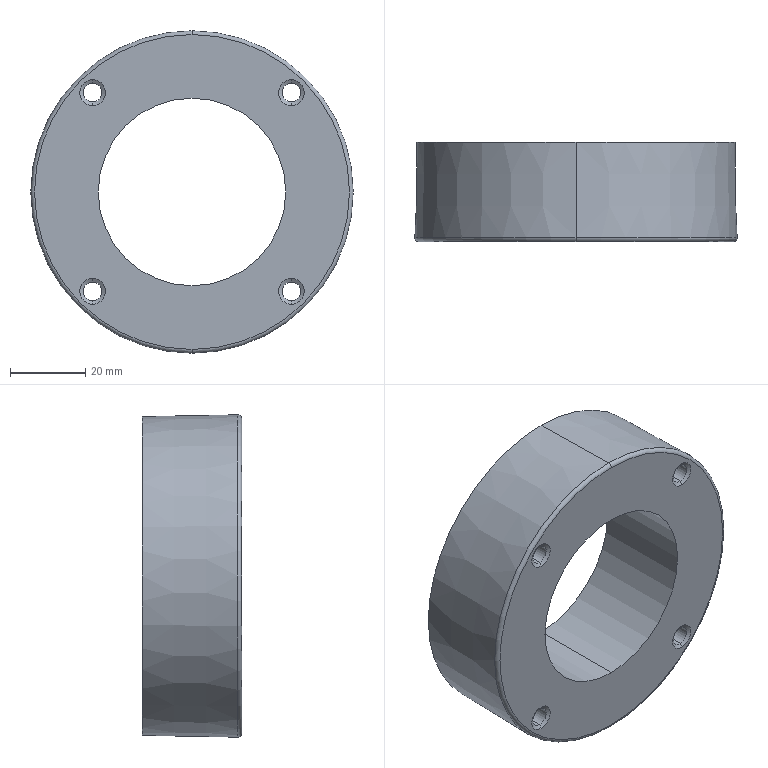Part | SolidWorks | features BaseBody 1 | 1 solid | 24 faces | box 85.962 x 26.5 x 85.962 mm | volume 97958 mm3 | cone 10 | cylinder 10 | torus 2 | plane 2 | commonest cylinder face diameters 5 x8 50 x2
STEP:
#1=CARTESIAN_POINT('',(33.,61.5,42.5));
#2=VERTEX_POINT('',#1);
#3=CARTESIAN_POINT('',(33.,61.5,-42.5));
#4=VERTEX_POINT('',#3);
#5=CARTESIAN_POINT('',(33.,61.5,0.));
#6=DIRECTION('',(0.,1.,0.));
#7=DIRECTION('',(0.,0.,-1.));
#8=AXIS2_PLACEMENT_3D('',#5,#6,#7);
#9=CIRCLE('',#8,42.5);
#10=EDGE_CURVE('',#2,#4,#9,.T.);
#11=ORIENTED_EDGE('',*,*,#10,.F.);
#12=CARTESIAN_POINT('',(33.,36.019,42.981));
#13=VERTEX_POINT('',#12);
#14=CARTESIAN_POINT('',(33.,36.019,42.981));
#15=DIRECTION('',(0.,-0.9998,0.01886));
#16=VECTOR('',#15,1000.);
#17=LINE('',#14,#16);
#18=EDGE_CURVE('',#2,#13,#17,.T.);
#19=ORIENTED_EDGE('',*,*,#18,.T.);
#20=CARTESIAN_POINT('',(33.,36.019,-42.981));
#21=VERTEX_POINT('',#20);
#22=CARTESIAN_POINT('',(33.,36.019,0.));
#23=DIRECTION('',(0.,1.,0.));
#24=DIRECTION('',(0.,0.,-1.));
#25=AXIS2_PLACEMENT_3D('',#22,#23,#24);
#26=CIRCLE('',#25,42.981);
#27=EDGE_CURVE('',#13,#21,#26,.T.);
#28=ORIENTED_EDGE('',*,*,#27,.T.);
#29=CARTESIAN_POINT('',(33.,36.019,-42.981));
#30=DIRECTION('',(0.,-0.9998,-0.01886));
#31=VECTOR('',#30,1000.);
#32=LINE('',#29,#31);
#33=EDGE_CURVE('',#4,#21,#32,.T.);
#34=ORIENTED_EDGE('',*,*,#33,.F.);
#35=EDGE_LOOP('',(#11,#19,#28,#34));
#36=FACE_OUTER_BOUND('',#35,.T.);
#37=CARTESIAN_POINT('',(33.,36.019,0.));
#38=DIRECTION('',(0.,-1.,0.));
#39=DIRECTION('',(0.,0.,-1.));
#40=AXIS2_PLACEMENT_3D('',#37,#38,#39);
#41=CONICAL_SURFACE('',#40,42.981,0.01887);
#42=ADVANCED_FACE('',(#36),#41,.T.);
#43=CARTESIAN_POINT('',(33.,61.5,25.));
#44=VERTEX_POINT('',#43);
#45=CARTESIAN_POINT('',(33.,61.5,-25.));
#46=VERTEX_POINT('',#45);
#47=CARTESIAN_POINT('',(33.,61.5,0.));
#48=DIRECTION('',(0.,-1.,0.));
#49=DIRECTION('',(0.,0.,-1.));
#50=AXIS2_PLACEMENT_3D('',#47,#48,#49);
#51=CIRCLE('',#50,25.);
#52=EDGE_CURVE('',#44,#46,#51,.T.);
#53=ORIENTED_EDGE('',*,*,#52,.F.);
#54=CARTESIAN_POINT('',(33.,35.,25.));
#55=VERTEX_POINT('',#54);
#56=CARTESIAN_POINT('',(33.,35.,25.));
#57=DIRECTION('',(0.,-1.,0.));
#58=VECTOR('',#57,1000.);
#59=LINE('',#56,#58);
#60=EDGE_CURVE('',#44,#55,#59,.T.);
#61=ORIENTED_EDGE('',*,*,#60,.T.);
#62=CARTESIAN_POINT('',(33.,35.,-25.));
#63=VERTEX_POINT('',#62);
#64=CARTESIAN_POINT('',(33.,35.,0.));
#65=DIRECTION('',(0.,1.,0.));
#66=DIRECTION('',(0.,0.,-1.));
#67=AXIS2_PLACEMENT_3D('',#64,#65,#66);
#68=CIRCLE('',#67,25.);
#69=EDGE_CURVE('',#63,#55,#68,.T.);
#70=ORIENTED_EDGE('',*,*,#69,.F.);
#71=CARTESIAN_POINT('',(33.,35.,-25.));
#72=DIRECTION('',(0.,-1.,0.));
#73=VECTOR('',#72,1000.);
#74=LINE('',#71,#73);
#75=EDGE_CURVE('',#46,#63,#74,.T.);
#76=ORIENTED_EDGE('',*,*,#75,.F.);
#77=EDGE_LOOP('',(#53,#61,#70,#76));
#78=FACE_OUTER_BOUND('',#77,.T.);
#79=CARTESIAN_POINT('',(33.,35.,0.));
#80=DIRECTION('',(0.,-1.,0.));
#81=DIRECTION('',(0.,0.,-1.));
#82=AXIS2_PLACEMENT_3D('',#79,#80,#81);
#83=CYLINDRICAL_SURFACE('',#82,25.);
#84=ADVANCED_FACE('',(#78),#83,.F.);
#85=CARTESIAN_POINT('',(59.5,61.5,29.));
#86=VERTEX_POINT('',#85);
#87=CARTESIAN_POINT('',(59.5,61.5,24.));
#88=VERTEX_POINT('',#87);
#89=CARTESIAN_POINT('',(59.5,61.5,26.5));
#90=DIRECTION('',(0.,-1.,0.));
#91=DIRECTION('',(0.,0.,-1.));
#92=AXIS2_PLACEMENT_3D('',#89,#90,#91);
#93=CIRCLE('',#92,2.5);
#94=EDGE_CURVE('',#86,#88,#93,.T.);
#95=ORIENTED_EDGE('',*,*,#94,.F.);
#96=CARTESIAN_POINT('',(59.5,35.548,29.));
#97=VERTEX_POINT('',#96);
#98=CARTESIAN_POINT('',(59.5,35.,29.));
#99=DIRECTION('',(0.,-1.,0.));
#100=VECTOR('',#99,1000.);
#101=LINE('',#98,#100);
#102=EDGE_CURVE('',#86,#97,#101,.T.);
#103=ORIENTED_EDGE('',*,*,#102,.T.);
#104=CARTESIAN_POINT('',(59.5,35.548,24.));
#105=VERTEX_POINT('',#104);
#106=CARTESIAN_POINT('',(59.5,35.548,26.5));
#107=DIRECTION('',(0.,1.,0.));
#108=DIRECTION('',(0.,0.,-1.));
#109=AXIS2_PLACEMENT_3D('',#106,#107,#108);
#110=CIRCLE('',#109,2.5);
#111=EDGE_CURVE('',#105,#97,#110,.T.);
#112=ORIENTED_EDGE('',*,*,#111,.F.);
#113=CARTESIAN_POINT('',(59.5,35.,24.));
#114=DIRECTION('',(0.,-1.,0.));
#115=VECTOR('',#114,1000.);
#116=LINE('',#113,#115);
#117=EDGE_CURVE('',#88,#105,#116,.T.);
#118=ORIENTED_EDGE('',*,*,#117,.F.);
#119=EDGE_LOOP('',(#95,#103,#112,#118));
#120=FACE_OUTER_BOUND('',#119,.T.);
#121=CARTESIAN_POINT('',(59.5,35.,26.5));
#122=DIRECTION('',(0.,-1.,0.));
#123=DIRECTION('',(0.,0.,-1.));
#124=AXIS2_PLACEMENT_3D('',#121,#122,#123);
#125=CYLINDRICAL_SURFACE('',#124,2.5);
#126=ADVANCED_FACE('',(#120),#125,.F.);
#127=CARTESIAN_POINT('',(59.5,61.5,-24.));
#128=VERTEX_POINT('',#127);
#129=CARTESIAN_POINT('',(59.5,61.5,-29.));
#130=VERTEX_POINT('',#129);
#131=CARTESIAN_POINT('',(59.5,61.5,-26.5));
#132=DIRECTION('',(0.,-1.,0.));
#133=DIRECTION('',(0.,0.,-1.));
#134=AXIS2_PLACEMENT_3D('',#131,#132,#133);
#135=CIRCLE('',#134,2.5);
#136=EDGE_CURVE('',#128,#130,#135,.T.);
#137=ORIENTED_EDGE('',*,*,#136,.F.);
#138=CARTESIAN_POINT('',(59.5,35.548,-24.));
#139=VERTEX_POINT('',#138);
#140=CARTESIAN_POINT('',(59.5,35.,-24.));
#141=DIRECTION('',(0.,-1.,0.));
#142=VECTOR('',#141,1000.);
#143=LINE('',#140,#142);
#144=EDGE_CURVE('',#128,#139,#143,.T.);
#145=ORIENTED_EDGE('',*,*,#144,.T.);
#146=CARTESIAN_POINT('',(59.5,35.548,-29.));
#147=VERTEX_POINT('',#146);
#148=CARTESIAN_POINT('',(59.5,35.548,-26.5));
#149=DIRECTION('',(0.,1.,0.));
#150=DIRECTION('',(0.,0.,-1.));
#151=AXIS2_PLACEMENT_3D('',#148,#149,#150);
#152=CIRCLE('',#151,2.5);
#153=EDGE_CURVE('',#147,#139,#152,.T.);
#154=ORIENTED_EDGE('',*,*,#153,.F.);
#155=CARTESIAN_POINT('',(59.5,35.,-29.));
#156=DIRECTION('',(0.,-1.,0.));
#157=VECTOR('',#156,1000.);
#158=LINE('',#155,#157);
#159=EDGE_CURVE('',#130,#147,#158,.T.);
#160=ORIENTED_EDGE('',*,*,#159,.F.);
#161=EDGE_LOOP('',(#137,#145,#154,#160));
#162=FACE_OUTER_BOUND('',#161,.T.);
#163=CARTESIAN_POINT('',(59.5,35.,-26.5));
#164=DIRECTION('',(0.,-1.,0.));
#165=DIRECTION('',(0.,0.,-1.));
#166=AXIS2_PLACEMENT_3D('',#163,#164,#165);
#167=CYLINDRICAL_SURFACE('',#166,2.5);
#168=ADVANCED_FACE('',(#162),#167,.F.);
#169=CARTESIAN_POINT('',(6.5,61.5,-24.));
#170=VERTEX_POINT('',#169);
#171=CARTESIAN_POINT('',(6.5,61.5,-29.));
#172=VERTEX_POINT('',#171);
#173=CARTESIAN_POINT('',(6.5,61.5,-26.5));
#174=DIRECTION('',(0.,-1.,0.));
#175=DIRECTION('',(0.,0.,-1.));
#176=AXIS2_PLACEMENT_3D('',#173,#174,#175);
#177=CIRCLE('',#176,2.5);
#178=EDGE_CURVE('',#170,#172,#177,.T.);
#179=ORIENTED_EDGE('',*,*,#178,.F.);
#180=CARTESIAN_POINT('',(6.5,35.548,-24.));
#181=VERTEX_POINT('',#180);
#182=CARTESIAN_POINT('',(6.5,35.,-24.));
#183=DIRECTION('',(0.,-1.,0.));
#184=VECTOR('',#183,1000.);
#185=LINE('',#182,#184);
#186=EDGE_CURVE('',#170,#181,#185,.T.);
#187=ORIENTED_EDGE('',*,*,#186,.T.);
#188=CARTESIAN_POINT('',(6.5,35.548,-29.));
#189=VERTEX_POINT('',#188);
#190=CARTESIAN_POINT('',(6.5,35.548,-26.5));
#191=DIRECTION('',(0.,1.,0.));
#192=DIRECTION('',(0.,0.,-1.));
#193=AXIS2_PLACEMENT_3D('',#190,#191,#192);
#194=CIRCLE('',#193,2.5);
#195=EDGE_CURVE('',#189,#181,#194,.T.);
#196=ORIENTED_EDGE('',*,*,#195,.F.);
#197=CARTESIAN_POINT('',(6.5,35.,-29.));
#198=DIRECTION('',(0.,-1.,0.));
#199=VECTOR('',#198,1000.);
#200=LINE('',#197,#199);
#201=EDGE_CURVE('',#172,#189,#200,.T.);
#202=ORIENTED_EDGE('',*,*,#201,.F.);
#203=EDGE_LOOP('',(#179,#187,#196,#202));
#204=FACE_OUTER_BOUND('',#203,.T.);
#205=CARTESIAN_POINT('',(6.5,35.,-26.5));
#206=DIRECTION('',(0.,-1.,0.));
#207=DIRECTION('',(0.,0.,-1.));
#208=AXIS2_PLACEMENT_3D('',#205,#206,#207);
#209=CYLINDRICAL_SURFACE('',#208,2.5);
#210=ADVANCED_FACE('',(#204),#209,.F.);
#211=CARTESIAN_POINT('',(6.5,61.5,29.));
#212=VERTEX_POINT('',#211);
#213=CARTESIAN_POINT('',(6.5,61.5,24.));
#214=VERTEX_POINT('',#213);
#215=CARTESIAN_POINT('',(6.5,61.5,26.5));
#216=DIRECTION('',(0.,-1.,0.));
#217=DIRECTION('',(0.,0.,-1.));
#218=AXIS2_PLACEMENT_3D('',#215,#216,#217);
#219=CIRCLE('',#218,2.5);
#220=EDGE_CURVE('',#212,#214,#219,.T.);
#221=ORIENTED_EDGE('',*,*,#220,.F.);
#222=CARTESIAN_POINT('',(6.5,35.548,29.));
#223=VERTEX_POINT('',#222);
#224=CARTESIAN_POINT('',(6.5,35.,29.));
#225=DIRECTION('',(0.,-1.,0.));
#226=VECTOR('',#225,1000.);
#227=LINE('',#224,#226);
#228=EDGE_CURVE('',#212,#223,#227,.T.);
#229=ORIENTED_EDGE('',*,*,#228,.T.);
#230=CARTESIAN_POINT('',(6.5,35.548,24.));
#231=VERTEX_POINT('',#230);
#232=CARTESIAN_POINT('',(6.5,35.548,26.5));
#233=DIRECTION('',(0.,1.,0.));
#234=DIRECTION('',(0.,0.,-1.));
#235=AXIS2_PLACEMENT_3D('',#232,#233,#234);
#236=CIRCLE('',#235,2.5);
#237=EDGE_CURVE('',#231,#223,#236,.T.);
#238=ORIENTED_EDGE('',*,*,#237,.F.);
#239=CARTESIAN_POINT('',(6.5,35.,24.));
#240=DIRECTION('',(0.,-1.,0.));
#241=VECTOR('',#240,1000.);
#242=LINE('',#239,#241);
#243=EDGE_CURVE('',#214,#231,#242,.T.);
#244=ORIENTED_EDGE('',*,*,#243,.F.);
#245=EDGE_LOOP('',(#221,#229,#238,#244));
#246=FACE_OUTER_BOUND('',#245,.T.);
#247=CARTESIAN_POINT('',(6.5,35.,26.5));
#248=DIRECTION('',(0.,-1.,0.));
#249=DIRECTION('',(0.,0.,-1.));
#250=AXIS2_PLACEMENT_3D('',#247,#248,#249);
#251=CYLINDRICAL_SURFACE('',#250,2.5);
#252=ADVANCED_FACE('',(#246),#251,.F.);
#253=ORIENTED_EDGE('',*,*,#27,.F.);
#254=CARTESIAN_POINT('',(33.,35.,41.981));
#255=VERTEX_POINT('',#254);
#256=CARTESIAN_POINT('',(33.,36.,41.981));
#257=DIRECTION('',(1.,0.,0.));
#258=DIRECTION('',(0.,0.,-1.));
#259=AXIS2_PLACEMENT_3D('',#256,#257,#258);
#260=CIRCLE('',#259,1.);
#261=EDGE_CURVE('',#13,#255,#260,.T.);
#262=ORIENTED_EDGE('',*,*,#261,.T.);
#263=CARTESIAN_POINT('',(33.,35.,-41.981));
#264=VERTEX_POINT('',#263);
#265=CARTESIAN_POINT('',(33.,35.,0.));
#266=DIRECTION('',(0.,1.,0.));
#267=DIRECTION('',(0.,0.,-1.));
#268=AXIS2_PLACEMENT_3D('',#265,#266,#267);
#269=CIRCLE('',#268,41.981);
#270=EDGE_CURVE('',#255,#264,#269,.T.);
#271=ORIENTED_EDGE('',*,*,#270,.T.);
#272=CARTESIAN_POINT('',(33.,36.,-41.981));
#273=DIRECTION('',(-1.,0.,0.));
#274=DIRECTION('',(0.,0.,1.));
#275=AXIS2_PLACEMENT_3D('',#272,#273,#274);
#276=CIRCLE('',#275,1.);
#277=EDGE_CURVE('',#21,#264,#276,.T.);
#278=ORIENTED_EDGE('',*,*,#277,.F.);
#279=EDGE_LOOP('',(#253,#262,#271,#278));
#280=FACE_OUTER_BOUND('',#279,.T.);
#281=CARTESIAN_POINT('',(33.,36.,0.));
#282=DIRECTION('',(0.,-1.,0.));
#283=DIRECTION('',(0.,0.,-1.));
#284=AXIS2_PLACEMENT_3D('',#281,#282,#283);
#285=TOROIDAL_SURFACE('',#284,41.981,1.);
#286=ADVANCED_FACE('',(#280),#285,.T.);
#287=ORIENTED_EDGE('',*,*,#111,.T.);
#288=CARTESIAN_POINT('',(59.5,35.,29.95));
#289=VERTEX_POINT('',#288);
#290=CARTESIAN_POINT('',(59.5,35.,29.95));
#291=DIRECTION('',(0.,-0.5,0.866));
#292=VECTOR('',#291,1000.);
#293=LINE('',#290,#292);
#294=EDGE_CURVE('',#97,#289,#293,.T.);
#295=ORIENTED_EDGE('',*,*,#294,.T.);
#296=CARTESIAN_POINT('',(59.5,35.,23.05));
#297=VERTEX_POINT('',#296);
#298=CARTESIAN_POINT('',(59.5,35.,26.5));
#299=DIRECTION('',(0.,-1.,0.));
#300=DIRECTION('',(0.,0.,-1.));
#301=AXIS2_PLACEMENT_3D('',#298,#299,#300);
#302=CIRCLE('',#301,3.45);
#303=EDGE_CURVE('',#289,#297,#302,.T.);
#304=ORIENTED_EDGE('',*,*,#303,.T.);
#305=CARTESIAN_POINT('',(59.5,35.,23.05));
#306=DIRECTION('',(0.,-0.5,-0.866));
#307=VECTOR('',#306,1000.);
#308=LINE('',#305,#307);
#309=EDGE_CURVE('',#105,#297,#308,.T.);
#310=ORIENTED_EDGE('',*,*,#309,.F.);
#311=EDGE_LOOP('',(#287,#295,#304,#310));
#312=FACE_OUTER_BOUND('',#311,.T.);
#313=CARTESIAN_POINT('',(59.5,35.,26.5));
#314=DIRECTION('',(0.,-1.,0.));
#315=DIRECTION('',(0.,0.,-1.));
#316=AXIS2_PLACEMENT_3D('',#313,#314,#315);
#317=CONICAL_SURFACE('',#316,3.45,1.047);
#318=ADVANCED_FACE('',(#312),#317,.F.);
#319=ORIENTED_EDGE('',*,*,#153,.T.);
#320=CARTESIAN_POINT('',(59.5,35.,-23.05));
#321=VERTEX_POINT('',#320);
#322=CARTESIAN_POINT('',(59.5,35.,-23.05));
#323=DIRECTION('',(0.,-0.5,0.866));
#324=VECTOR('',#323,1000.);
#325=LINE('',#322,#324);
#326=EDGE_CURVE('',#139,#321,#325,.T.);
#327=ORIENTED_EDGE('',*,*,#326,.T.);
#328=CARTESIAN_POINT('',(59.5,35.,-29.95));
#329=VERTEX_POINT('',#328);
#330=CARTESIAN_POINT('',(59.5,35.,-26.5));
#331=DIRECTION('',(0.,-1.,0.));
#332=DIRECTION('',(0.,0.,-1.));
#333=AXIS2_PLACEMENT_3D('',#330,#331,#332);
#334=CIRCLE('',#333,3.45);
#335=EDGE_CURVE('',#321,#329,#334,.T.);
#336=ORIENTED_EDGE('',*,*,#335,.T.);
#337=CARTESIAN_POINT('',(59.5,35.,-29.95));
#338=DIRECTION('',(0.,-0.5,-0.866));
#339=VECTOR('',#338,1000.);
#340=LINE('',#337,#339);
#341=EDGE_CURVE('',#147,#329,#340,.T.);
#342=ORIENTED_EDGE('',*,*,#341,.F.);
#343=EDGE_LOOP('',(#319,#327,#336,#342));
#344=FACE_OUTER_BOUND('',#343,.T.);
#345=CARTESIAN_POINT('',(59.5,35.,-26.5));
#346=DIRECTION('',(0.,-1.,0.));
#347=DIRECTION('',(0.,0.,-1.));
#348=AXIS2_PLACEMENT_3D('',#345,#346,#347);
#349=CONICAL_SURFACE('',#348,3.45,1.047);
#350=ADVANCED_FACE('',(#344),#349,.F.);
#351=ORIENTED_EDGE('',*,*,#195,.T.);
#352=CARTESIAN_POINT('',(6.5,35.,-23.05));
#353=VERTEX_POINT('',#352);
#354=CARTESIAN_POINT('',(6.5,35.,-23.05));
#355=DIRECTION('',(0.,-0.5,0.866));
#356=VECTOR('',#355,1000.);
#357=LINE('',#354,#356);
#358=EDGE_CURVE('',#181,#353,#357,.T.);
#359=ORIENTED_EDGE('',*,*,#358,.T.);
#360=CARTESIAN_POINT('',(6.5,35.,-29.95));
#361=VERTEX_POINT('',#360);
#362=CARTESIAN_POINT('',(6.5,35.,-26.5));
#363=DIRECTION('',(0.,-1.,0.));
#364=DIRECTION('',(0.,0.,-1.));
#365=AXIS2_PLACEMENT_3D('',#362,#363,#364);
#366=CIRCLE('',#365,3.45);
#367=EDGE_CURVE('',#353,#361,#366,.T.);
#368=ORIENTED_EDGE('',*,*,#367,.T.);
#369=CARTESIAN_POINT('',(6.5,35.,-29.95));
#370=DIRECTION('',(0.,-0.5,-0.866));
#371=VECTOR('',#370,1000.);
#372=LINE('',#369,#371);
#373=EDGE_CURVE('',#189,#361,#372,.T.);
#374=ORIENTED_EDGE('',*,*,#373,.F.);
#375=EDGE_LOOP('',(#351,#359,#368,#374));
#376=FACE_OUTER_BOUND('',#375,.T.);
#377=CARTESIAN_POINT('',(6.5,35.,-26.5));
#378=DIRECTION('',(0.,-1.,0.));
#379=DIRECTION('',(0.,0.,-1.));
#380=AXIS2_PLACEMENT_3D('',#377,#378,#379);
#381=CONICAL_SURFACE('',#380,3.45,1.047);
#382=ADVANCED_FACE('',(#376),#381,.F.);
#383=ORIENTED_EDGE('',*,*,#237,.T.);
#384=CARTESIAN_POINT('',(6.5,35.,29.95));
#385=VERTEX_POINT('',#384);
#386=CARTESIAN_POINT('',(6.5,35.,29.95));
#387=DIRECTION('',(0.,-0.5,0.866));
#388=VECTOR('',#387,1000.);
#389=LINE('',#386,#388);
#390=EDGE_CURVE('',#223,#385,#389,.T.);
#391=ORIENTED_EDGE('',*,*,#390,.T.);
#392=CARTESIAN_POINT('',(6.5,35.,23.05));
#393=VERTEX_POINT('',#392);
#394=CARTESIAN_POINT('',(6.5,35.,26.5));
#395=DIRECTION('',(0.,-1.,0.));
#396=DIRECTION('',(0.,0.,-1.));
#397=AXIS2_PLACEMENT_3D('',#394,#395,#396);
#398=CIRCLE('',#397,3.45);
#399=EDGE_CURVE('',#385,#393,#398,.T.);
#400=ORIENTED_EDGE('',*,*,#399,.T.);
#401=CARTESIAN_POINT('',(6.5,35.,23.05));
#402=DIRECTION('',(0.,-0.5,-0.866));
#403=VECTOR('',#402,1000.);
#404=LINE('',#401,#403);
#405=EDGE_CURVE('',#231,#393,#404,.T.);
#406=ORIENTED_EDGE('',*,*,#405,.F.);
#407=EDGE_LOOP('',(#383,#391,#400,#406));
#408=FACE_OUTER_BOUND('',#407,.T.);
#409=CARTESIAN_POINT('',(6.5,35.,26.5));
#410=DIRECTION('',(0.,-1.,0.));
#411=DIRECTION('',(0.,0.,-1.));
#412=AXIS2_PLACEMENT_3D('',#409,#410,#411);
#413=CONICAL_SURFACE('',#412,3.45,1.047);
#414=ADVANCED_FACE('',(#408),#413,.F.);
#415=CARTESIAN_POINT('',(33.,61.5,0.));
#416=DIRECTION('',(0.,1.,0.));
#417=DIRECTION('',(0.,0.,-1.));
#418=AXIS2_PLACEMENT_3D('',#415,#416,#417);
#419=CIRCLE('',#418,42.5);
#420=EDGE_CURVE('',#4,#2,#419,.T.);
#421=ORIENTED_EDGE('',*,*,#420,.T.);
#422=ORIENTED_EDGE('',*,*,#10,.T.);
#423=EDGE_LOOP('',(#421,#422));
#424=FACE_OUTER_BOUND('',#423,.T.);
#425=CARTESIAN_POINT('',(33.,61.5,0.));
#426=DIRECTION('',(0.,-1.,0.));
#427=DIRECTION('',(0.,0.,-1.));
#428=AXIS2_PLACEMENT_3D('',#425,#426,#427);
#429=CIRCLE('',#428,25.);
#430=EDGE_CURVE('',#46,#44,#429,.T.);
#431=ORIENTED_EDGE('',*,*,#430,.T.);
#432=ORIENTED_EDGE('',*,*,#52,.T.);
#433=EDGE_LOOP('',(#431,#432));
#434=FACE_BOUND('',#433,.T.);
#435=CARTESIAN_POINT('',(59.5,61.5,26.5));
#436=DIRECTION('',(0.,-1.,0.));
#437=DIRECTION('',(0.,0.,-1.));
#438=AXIS2_PLACEMENT_3D('',#435,#436,#437);
#439=CIRCLE('',#438,2.5);
#440=EDGE_CURVE('',#88,#86,#439,.T.);
#441=ORIENTED_EDGE('',*,*,#440,.T.);
#442=ORIENTED_EDGE('',*,*,#94,.T.);
#443=EDGE_LOOP('',(#441,#442));
#444=FACE_BOUND('',#443,.T.);
#445=CARTESIAN_POINT('',(59.5,61.5,-26.5));
#446=DIRECTION('',(0.,-1.,0.));
#447=DIRECTION('',(0.,0.,-1.));
#448=AXIS2_PLACEMENT_3D('',#445,#446,#447);
#449=CIRCLE('',#448,2.5);
#450=EDGE_CURVE('',#130,#128,#449,.T.);
#451=ORIENTED_EDGE('',*,*,#450,.T.);
#452=ORIENTED_EDGE('',*,*,#136,.T.);
#453=EDGE_LOOP('',(#451,#452));
#454=FACE_BOUND('',#453,.T.);
#455=CARTESIAN_POINT('',(6.5,61.5,-26.5));
#456=DIRECTION('',(0.,-1.,0.));
#457=DIRECTION('',(0.,0.,-1.));
#458=AXIS2_PLACEMENT_3D('',#455,#456,#457);
#459=CIRCLE('',#458,2.5);
#460=EDGE_CURVE('',#172,#170,#459,.T.);
#461=ORIENTED_EDGE('',*,*,#460,.T.);
#462=ORIENTED_EDGE('',*,*,#178,.T.);
#463=EDGE_LOOP('',(#461,#462));
#464=FACE_BOUND('',#463,.T.);
#465=CARTESIAN_POINT('',(6.5,61.5,26.5));
#466=DIRECTION('',(0.,-1.,0.));
#467=DIRECTION('',(0.,0.,-1.));
#468=AXIS2_PLACEMENT_3D('',#465,#466,#467);
#469=CIRCLE('',#468,2.5);
#470=EDGE_CURVE('',#214,#212,#469,.T.);
#471=ORIENTED_EDGE('',*,*,#470,.T.);
#472=ORIENTED_EDGE('',*,*,#220,.T.);
#473=EDGE_LOOP('',(#471,#472));
#474=FACE_BOUND('',#473,.T.);
#475=CARTESIAN_POINT('',(11.75,61.5,0.));
#476=DIRECTION('',(0.,1.,0.));
#477=DIRECTION('',(0.,0.,1.));
#478=AXIS2_PLACEMENT_3D('',#475,#476,#477);
#479=PLANE('',#478);
#480=ADVANCED_FACE('',(#424,#434,#444,#454,#464,#474),#479,.T.);
#481=ORIENTED_EDGE('',*,*,#18,.F.);
#482=ORIENTED_EDGE('',*,*,#420,.F.);
#483=ORIENTED_EDGE('',*,*,#33,.T.);
#484=CARTESIAN_POINT('',(33.,36.019,0.));
#485=DIRECTION('',(0.,1.,0.));
#486=DIRECTION('',(0.,0.,-1.));
#487=AXIS2_PLACEMENT_3D('',#484,#485,#486);
#488=CIRCLE('',#487,42.981);
#489=EDGE_CURVE('',#21,#13,#488,.T.);
#490=ORIENTED_EDGE('',*,*,#489,.T.);
#491=EDGE_LOOP('',(#481,#482,#483,#490));
#492=FACE_OUTER_BOUND('',#491,.T.);
#493=CARTESIAN_POINT('',(33.,36.019,0.));
#494=DIRECTION('',(0.,-1.,0.));
#495=DIRECTION('',(0.,0.,-1.));
#496=AXIS2_PLACEMENT_3D('',#493,#494,#495);
#497=CONICAL_SURFACE('',#496,42.981,0.01887);
#498=ADVANCED_FACE('',(#492),#497,.T.);
#499=ORIENTED_EDGE('',*,*,#60,.F.);
#500=ORIENTED_EDGE('',*,*,#430,.F.);
#501=ORIENTED_EDGE('',*,*,#75,.T.);
#502=CARTESIAN_POINT('',(33.,35.,0.));
#503=DIRECTION('',(0.,1.,0.));
#504=DIRECTION('',(0.,0.,-1.));
#505=AXIS2_PLACEMENT_3D('',#502,#503,#504);
#506=CIRCLE('',#505,25.);
#507=EDGE_CURVE('',#55,#63,#506,.T.);
#508=ORIENTED_EDGE('',*,*,#507,.F.);
#509=EDGE_LOOP('',(#499,#500,#501,#508));
#510=FACE_OUTER_BOUND('',#509,.T.);
#511=CARTESIAN_POINT('',(33.,35.,0.));
#512=DIRECTION('',(0.,-1.,0.));
#513=DIRECTION('',(0.,0.,-1.));
#514=AXIS2_PLACEMENT_3D('',#511,#512,#513);
#515=CYLINDRICAL_SURFACE('',#514,25.);
#516=ADVANCED_FACE('',(#510),#515,.F.);
#517=ORIENTED_EDGE('',*,*,#102,.F.);
#518=ORIENTED_EDGE('',*,*,#440,.F.);
#519=ORIENTED_EDGE('',*,*,#117,.T.);
#520=CARTESIAN_POINT('',(59.5,35.548,26.5));
#521=DIRECTION('',(0.,1.,0.));
#522=DIRECTION('',(0.,0.,-1.));
#523=AXIS2_PLACEMENT_3D('',#520,#521,#522);
#524=CIRCLE('',#523,2.5);
#525=EDGE_CURVE('',#97,#105,#524,.T.);
#526=ORIENTED_EDGE('',*,*,#525,.F.);
#527=EDGE_LOOP('',(#517,#518,#519,#526));
#528=FACE_OUTER_BOUND('',#527,.T.);
#529=CARTESIAN_POINT('',(59.5,35.,26.5));
#530=DIRECTION('',(0.,-1.,0.));
#531=DIRECTION('',(0.,0.,-1.));
#532=AXIS2_PLACEMENT_3D('',#529,#530,#531);
#533=CYLINDRICAL_SURFACE('',#532,2.5);
#534=ADVANCED_FACE('',(#528),#533,.F.);
#535=ORIENTED_EDGE('',*,*,#144,.F.);
#536=ORIENTED_EDGE('',*,*,#450,.F.);
#537=ORIENTED_EDGE('',*,*,#159,.T.);
#538=CARTESIAN_POINT('',(59.5,35.548,-26.5));
#539=DIRECTION('',(0.,1.,0.));
#540=DIRECTION('',(0.,0.,-1.));
#541=AXIS2_PLACEMENT_3D('',#538,#539,#540);
#542=CIRCLE('',#541,2.5);
#543=EDGE_CURVE('',#139,#147,#542,.T.);
#544=ORIENTED_EDGE('',*,*,#543,.F.);
#545=EDGE_LOOP('',(#535,#536,#537,#544));
#546=FACE_OUTER_BOUND('',#545,.T.);
#547=CARTESIAN_POINT('',(59.5,35.,-26.5));
#548=DIRECTION('',(0.,-1.,0.));
#549=DIRECTION('',(0.,0.,-1.));
#550=AXIS2_PLACEMENT_3D('',#547,#548,#549);
#551=CYLINDRICAL_SURFACE('',#550,2.5);
#552=ADVANCED_FACE('',(#546),#551,.F.);
#553=ORIENTED_EDGE('',*,*,#186,.F.);
#554=ORIENTED_EDGE('',*,*,#460,.F.);
#555=ORIENTED_EDGE('',*,*,#201,.T.);
#556=CARTESIAN_POINT('',(6.5,35.548,-26.5));
#557=DIRECTION('',(0.,1.,0.));
#558=DIRECTION('',(0.,0.,-1.));
#559=AXIS2_PLACEMENT_3D('',#556,#557,#558);
#560=CIRCLE('',#559,2.5);
#561=EDGE_CURVE('',#181,#189,#560,.T.);
#562=ORIENTED_EDGE('',*,*,#561,.F.);
#563=EDGE_LOOP('',(#553,#554,#555,#562));
#564=FACE_OUTER_BOUND('',#563,.T.);
#565=CARTESIAN_POINT('',(6.5,35.,-26.5));
#566=DIRECTION('',(0.,-1.,0.));
#567=DIRECTION('',(0.,0.,-1.));
#568=AXIS2_PLACEMENT_3D('',#565,#566,#567);
#569=CYLINDRICAL_SURFACE('',#568,2.5);
#570=ADVANCED_FACE('',(#564),#569,.F.);
#571=ORIENTED_EDGE('',*,*,#228,.F.);
#572=ORIENTED_EDGE('',*,*,#470,.F.);
#573=ORIENTED_EDGE('',*,*,#243,.T.);
#574=CARTESIAN_POINT('',(6.5,35.548,26.5));
#575=DIRECTION('',(0.,1.,0.));
#576=DIRECTION('',(0.,0.,-1.));
#577=AXIS2_PLACEMENT_3D('',#574,#575,#576);
#578=CIRCLE('',#577,2.5);
#579=EDGE_CURVE('',#223,#231,#578,.T.);
#580=ORIENTED_EDGE('',*,*,#579,.F.);
#581=EDGE_LOOP('',(#571,#572,#573,#580));
#582=FACE_OUTER_BOUND('',#581,.T.);
#583=CARTESIAN_POINT('',(6.5,35.,26.5));
#584=DIRECTION('',(0.,-1.,0.));
#585=DIRECTION('',(0.,0.,-1.));
#586=AXIS2_PLACEMENT_3D('',#583,#584,#585);
#587=CYLINDRICAL_SURFACE('',#586,2.5);
#588=ADVANCED_FACE('',(#582),#587,.F.);
#589=ORIENTED_EDGE('',*,*,#261,.F.);
#590=ORIENTED_EDGE('',*,*,#489,.F.);
#591=ORIENTED_EDGE('',*,*,#277,.T.);
#592=CARTESIAN_POINT('',(33.,35.,0.));
#593=DIRECTION('',(0.,1.,0.));
#594=DIRECTION('',(0.,0.,-1.));
#595=AXIS2_PLACEMENT_3D('',#592,#593,#594);
#596=CIRCLE('',#595,41.981);
#597=EDGE_CURVE('',#264,#255,#596,.T.);
#598=ORIENTED_EDGE('',*,*,#597,.T.);
#599=EDGE_LOOP('',(#589,#590,#591,#598));
#600=FACE_OUTER_BOUND('',#599,.T.);
#601=CARTESIAN_POINT('',(33.,36.,0.));
#602=DIRECTION('',(0.,-1.,0.));
#603=DIRECTION('',(0.,0.,-1.));
#604=AXIS2_PLACEMENT_3D('',#601,#602,#603);
#605=TOROIDAL_SURFACE('',#604,41.981,1.);
#606=ADVANCED_FACE('',(#600),#605,.T.);
#607=ORIENTED_EDGE('',*,*,#597,.F.);
#608=ORIENTED_EDGE('',*,*,#270,.F.);
#609=EDGE_LOOP('',(#607,#608));
#610=FACE_OUTER_BOUND('',#609,.T.);
#611=CARTESIAN_POINT('',(59.5,35.,26.5));
#612=DIRECTION('',(0.,-1.,0.));
#613=DIRECTION('',(0.,0.,-1.));
#614=AXIS2_PLACEMENT_3D('',#611,#612,#613);
#615=CIRCLE('',#614,3.45);
#616=EDGE_CURVE('',#297,#289,#615,.T.);
#617=ORIENTED_EDGE('',*,*,#616,.F.);
#618=ORIENTED_EDGE('',*,*,#303,.F.);
#619=EDGE_LOOP('',(#617,#618));
#620=FACE_BOUND('',#619,.T.);
#621=CARTESIAN_POINT('',(6.5,35.,-26.5));
#622=DIRECTION('',(0.,-1.,0.));
#623=DIRECTION('',(0.,0.,-1.));
#624=AXIS2_PLACEMENT_3D('',#621,#622,#623);
#625=CIRCLE('',#624,3.45);
#626=EDGE_CURVE('',#361,#353,#625,.T.);
#627=ORIENTED_EDGE('',*,*,#626,.F.);
#628=ORIENTED_EDGE('',*,*,#367,.F.);
#629=EDGE_LOOP('',(#627,#628));
#630=FACE_BOUND('',#629,.T.);
#631=ORIENTED_EDGE('',*,*,#69,.T.);
#632=ORIENTED_EDGE('',*,*,#507,.T.);
#633=EDGE_LOOP('',(#631,#632));
#634=FACE_BOUND('',#633,.T.);
#635=CARTESIAN_POINT('',(6.5,35.,26.5));
#636=DIRECTION('',(0.,-1.,0.));
#637=DIRECTION('',(0.,0.,-1.));
#638=AXIS2_PLACEMENT_3D('',#635,#636,#637);
#639=CIRCLE('',#638,3.45);
#640=EDGE_CURVE('',#393,#385,#639,.T.);
#641=ORIENTED_EDGE('',*,*,#640,.F.);
#642=ORIENTED_EDGE('',*,*,#399,.F.);
#643=EDGE_LOOP('',(#641,#642));
#644=FACE_BOUND('',#643,.T.);
#645=CARTESIAN_POINT('',(59.5,35.,-26.5));
#646=DIRECTION('',(0.,-1.,0.));
#647=DIRECTION('',(0.,0.,-1.));
#648=AXIS2_PLACEMENT_3D('',#645,#646,#647);
#649=CIRCLE('',#648,3.45);
#650=EDGE_CURVE('',#329,#321,#649,.T.);
#651=ORIENTED_EDGE('',*,*,#650,.F.);
#652=ORIENTED_EDGE('',*,*,#335,.F.);
#653=EDGE_LOOP('',(#651,#652));
#654=FACE_BOUND('',#653,.T.);
#655=CARTESIAN_POINT('',(11.5,35.,0.));
#656=DIRECTION('',(0.,1.,0.));
#657=DIRECTION('',(0.,0.,1.));
#658=AXIS2_PLACEMENT_3D('',#655,#656,#657);
#659=PLANE('',#658);
#660=ADVANCED_FACE('',(#610,#620,#630,#634,#644,#654),#659,.F.);
#661=ORIENTED_EDGE('',*,*,#294,.F.);
#662=ORIENTED_EDGE('',*,*,#525,.T.);
#663=ORIENTED_EDGE('',*,*,#309,.T.);
#664=ORIENTED_EDGE('',*,*,#616,.T.);
#665=EDGE_LOOP('',(#661,#662,#663,#664));
#666=FACE_OUTER_BOUND('',#665,.T.);
#667=CARTESIAN_POINT('',(59.5,35.,26.5));
#668=DIRECTION('',(0.,-1.,0.));
#669=DIRECTION('',(0.,0.,-1.));
#670=AXIS2_PLACEMENT_3D('',#667,#668,#669);
#671=CONICAL_SURFACE('',#670,3.45,1.047);
#672=ADVANCED_FACE('',(#666),#671,.F.);
#673=ORIENTED_EDGE('',*,*,#326,.F.);
#674=ORIENTED_EDGE('',*,*,#543,.T.);
#675=ORIENTED_EDGE('',*,*,#341,.T.);
#676=ORIENTED_EDGE('',*,*,#650,.T.);
#677=EDGE_LOOP('',(#673,#674,#675,#676));
#678=FACE_OUTER_BOUND('',#677,.T.);
#679=CARTESIAN_POINT('',(59.5,35.,-26.5));
#680=DIRECTION('',(0.,-1.,0.));
#681=DIRECTION('',(0.,0.,-1.));
#682=AXIS2_PLACEMENT_3D('',#679,#680,#681);
#683=CONICAL_SURFACE('',#682,3.45,1.047);
#684=ADVANCED_FACE('',(#678),#683,.F.);
#685=ORIENTED_EDGE('',*,*,#358,.F.);
#686=ORIENTED_EDGE('',*,*,#561,.T.);
#687=ORIENTED_EDGE('',*,*,#373,.T.);
#688=ORIENTED_EDGE('',*,*,#626,.T.);
#689=EDGE_LOOP('',(#685,#686,#687,#688));
#690=FACE_OUTER_BOUND('',#689,.T.);
#691=CARTESIAN_POINT('',(6.5,35.,-26.5));
#692=DIRECTION('',(0.,-1.,0.));
#693=DIRECTION('',(0.,0.,-1.));
#694=AXIS2_PLACEMENT_3D('',#691,#692,#693);
#695=CONICAL_SURFACE('',#694,3.45,1.047);
#696=ADVANCED_FACE('',(#690),#695,.F.);
#697=ORIENTED_EDGE('',*,*,#390,.F.);
#698=ORIENTED_EDGE('',*,*,#579,.T.);
#699=ORIENTED_EDGE('',*,*,#405,.T.);
#700=ORIENTED_EDGE('',*,*,#640,.T.);
#701=EDGE_LOOP('',(#697,#698,#699,#700));
#702=FACE_OUTER_BOUND('',#701,.T.);
#703=CARTESIAN_POINT('',(6.5,35.,26.5));
#704=DIRECTION('',(0.,-1.,0.));
#705=DIRECTION('',(0.,0.,-1.));
#706=AXIS2_PLACEMENT_3D('',#703,#704,#705);
#707=CONICAL_SURFACE('',#706,3.45,1.047);
#708=ADVANCED_FACE('',(#702),#707,.F.);
#709=CLOSED_SHELL('',(#42,#84,#126,#168,#210,#252,#286,#318,#350,#382,#414,#480,#498,#516,#534,#552,#570,#588,#606,#660,#672,#684,#696,#708));
#710=MANIFOLD_SOLID_BREP('',#709);
#711=CARTESIAN_POINT('',(0.,0.,0.));
#712=DIRECTION('',(0.,0.,1.));
#713=DIRECTION('',(1.,0.,0.));
#714=AXIS2_PLACEMENT_3D('',#711,#712,#713);
#715=(LENGTH_UNIT()NAMED_UNIT(*)SI_UNIT(.MILLI.,.METRE.));
#716=UNCERTAINTY_MEASURE_WITH_UNIT(LENGTH_MEASURE(0.00001),#715,'','');
#717=(NAMED_UNIT(*)PLANE_ANGLE_UNIT()SI_UNIT($,.RADIAN.));
#718=(NAMED_UNIT(*)SI_UNIT($,.STERADIAN.)SOLID_ANGLE_UNIT());
#719=(GEOMETRIC_REPRESENTATION_CONTEXT(3)GLOBAL_UNCERTAINTY_ASSIGNED_CONTEXT((#716))GLOBAL_UNIT_ASSIGNED_CONTEXT((#715,#717,#718))REPRESENTATION_CONTEXT('',''));
#720=ADVANCED_BREP_SHAPE_REPRESENTATION('',(#710,#714),#719);